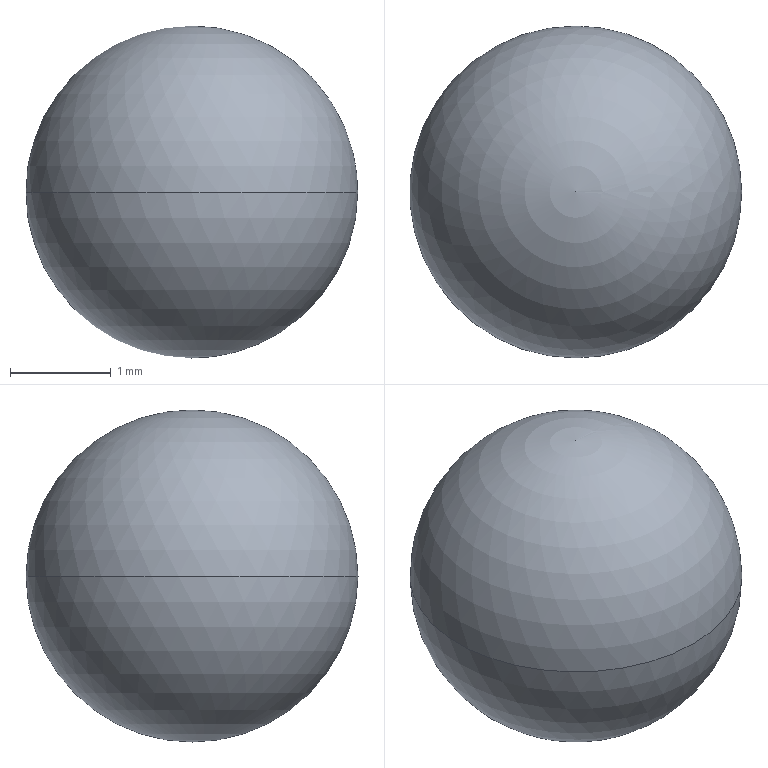Part | SolidWorks | features Revolution 1 | 1 solid | 2 faces | box 3.3 x 3.3 x 3.3 mm | volume 18.817 mm3 | sphere 2
STEP:
#1=CARTESIAN_POINT('',(0.,-1.65,0.));
#2=VERTEX_POINT('',#1);
#3=CARTESIAN_POINT('',(0.,1.65,0.));
#4=VERTEX_POINT('',#3);
#5=CARTESIAN_POINT('',(0.,0.,0.));
#6=DIRECTION('',(0.,0.,1.));
#7=DIRECTION('',(1.,0.,0.));
#8=AXIS2_PLACEMENT_3D('',#5,#6,#7);
#9=CIRCLE('',#8,1.65);
#10=EDGE_CURVE('',#2,#4,#9,.T.);
#11=ORIENTED_EDGE('',*,*,#10,.F.);
#12=CARTESIAN_POINT('',(0.,0.,0.));
#13=DIRECTION('',(0.,0.,-1.));
#14=DIRECTION('',(-1.,0.,0.));
#15=AXIS2_PLACEMENT_3D('',#12,#13,#14);
#16=CIRCLE('',#15,1.65);
#17=EDGE_CURVE('',#2,#4,#16,.T.);
#18=ORIENTED_EDGE('',*,*,#17,.T.);
#19=EDGE_LOOP('',(#11,#18));
#20=FACE_OUTER_BOUND('',#19,.T.);
#21=CARTESIAN_POINT('',(0.,0.,0.));
#22=DIRECTION('',(0.,0.,-1.));
#23=DIRECTION('',(1.,0.,0.));
#24=AXIS2_PLACEMENT_3D('',#21,#22,#23);
#25=SPHERICAL_SURFACE('',#24,1.65);
#26=ADVANCED_FACE('',(#20),#25,.T.);
#27=ORIENTED_EDGE('',*,*,#17,.F.);
#28=ORIENTED_EDGE('',*,*,#10,.T.);
#29=EDGE_LOOP('',(#27,#28));
#30=FACE_OUTER_BOUND('',#29,.T.);
#31=CARTESIAN_POINT('',(0.,0.,0.));
#32=DIRECTION('',(0.,0.,-1.));
#33=DIRECTION('',(1.,0.,0.));
#34=AXIS2_PLACEMENT_3D('',#31,#32,#33);
#35=SPHERICAL_SURFACE('',#34,1.65);
#36=ADVANCED_FACE('',(#30),#35,.T.);
#37=CLOSED_SHELL('',(#26,#36));
#38=MANIFOLD_SOLID_BREP('',#37);
#39=CARTESIAN_POINT('',(0.,0.,0.));
#40=DIRECTION('',(0.,0.,1.));
#41=DIRECTION('',(1.,0.,0.));
#42=AXIS2_PLACEMENT_3D('',#39,#40,#41);
#43=(LENGTH_UNIT()NAMED_UNIT(*)SI_UNIT(.MILLI.,.METRE.));
#44=UNCERTAINTY_MEASURE_WITH_UNIT(LENGTH_MEASURE(0.00001),#43,'','');
#45=(NAMED_UNIT(*)PLANE_ANGLE_UNIT()SI_UNIT($,.RADIAN.));
#46=(NAMED_UNIT(*)SI_UNIT($,.STERADIAN.)SOLID_ANGLE_UNIT());
#47=(GEOMETRIC_REPRESENTATION_CONTEXT(3)GLOBAL_UNCERTAINTY_ASSIGNED_CONTEXT((#44))GLOBAL_UNIT_ASSIGNED_CONTEXT((#43,#45,#46))REPRESENTATION_CONTEXT('',''));
#48=ADVANCED_BREP_SHAPE_REPRESENTATION('',(#38,#42),#47);